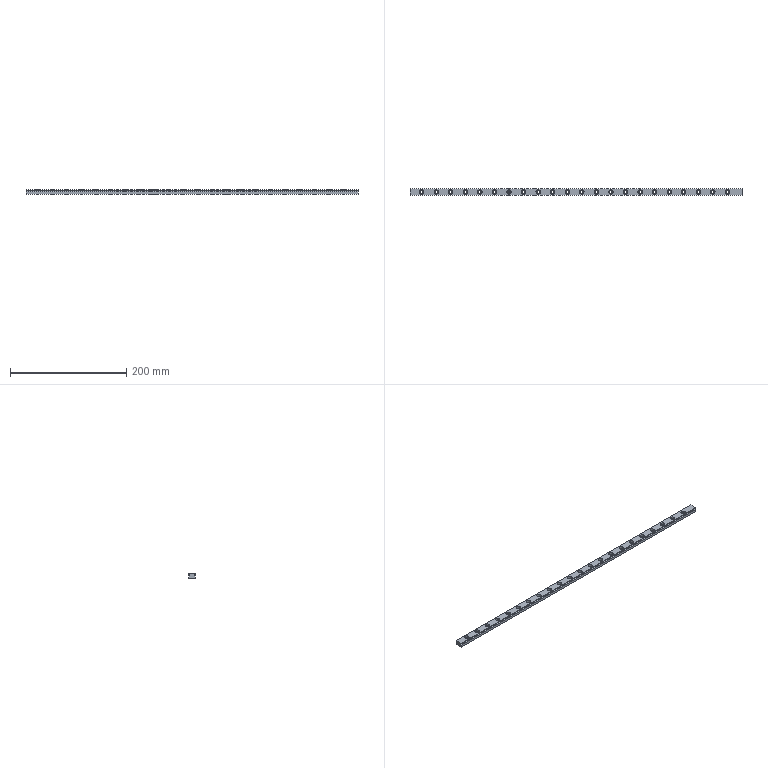Part | SolidWorks | features BaseBody 1 | 1 solid | 120 faces | box 570 x 12 x 8 mm | volume 46406 mm3 | cylinder 90 | plane 30 | commonest cylinder face diameters 4.5 x44 7.5 x44 2.6 x2